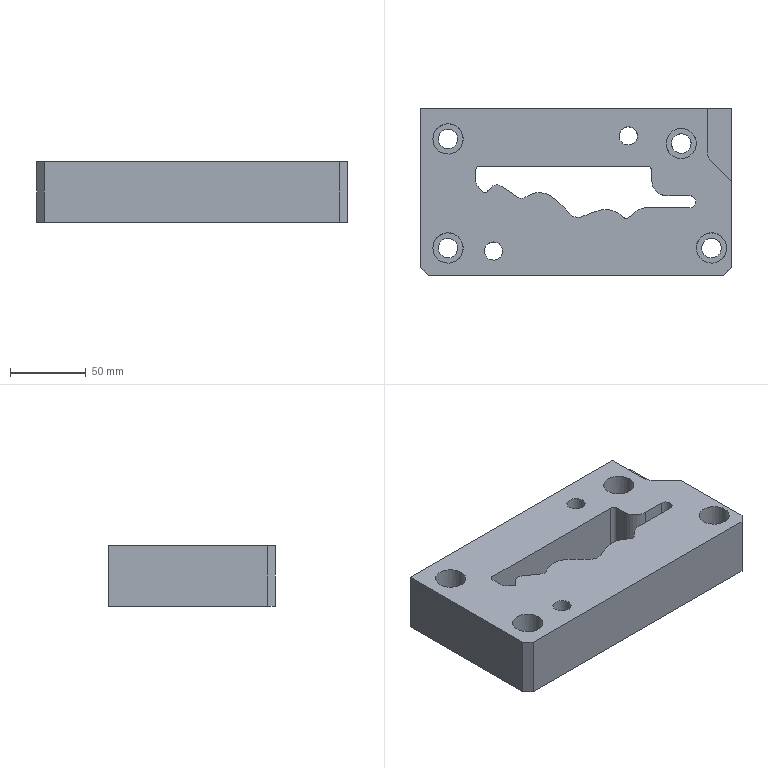Part | STEP file | gslz 2016.10.28-13_id174_x_t | 1 solid | 54 faces | box 205 x 110 x 40 mm | volume 725690 mm3 | plane 28 | cylinder 26 | commonest cylinder face diameters 20 x6 4 x4 13 x4 10 x3 12 x2 6 x1